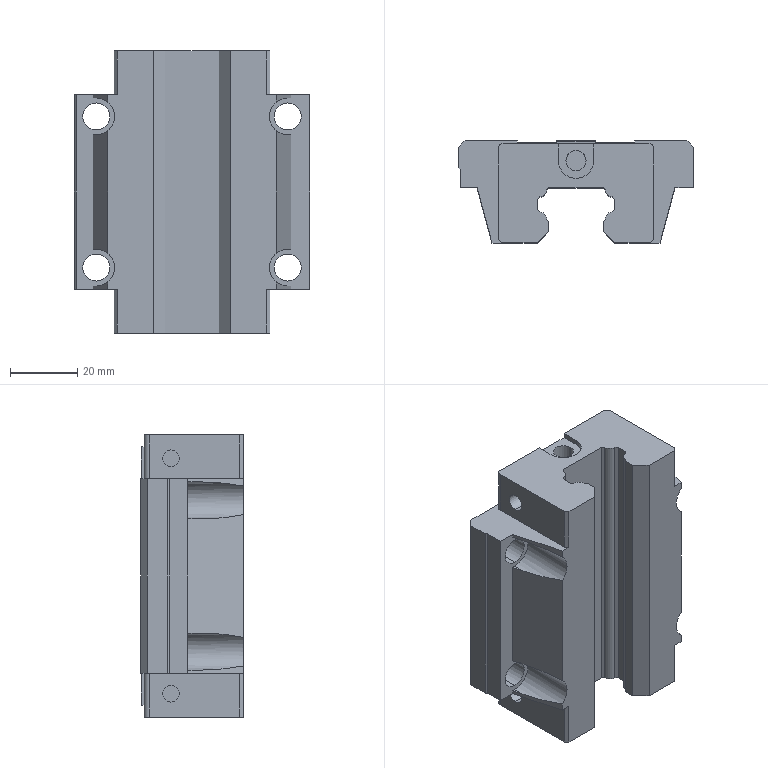Part | SolidWorks | features BaseBody 1 | 1 solid | 137 faces | box 70 x 30.5 x 84 mm | volume 110295 mm3 | plane 92 | cylinder 45 | commonest cylinder face diameters 5 x8 8 x8 1 x7 3 x4 4.6 x4 6 x4